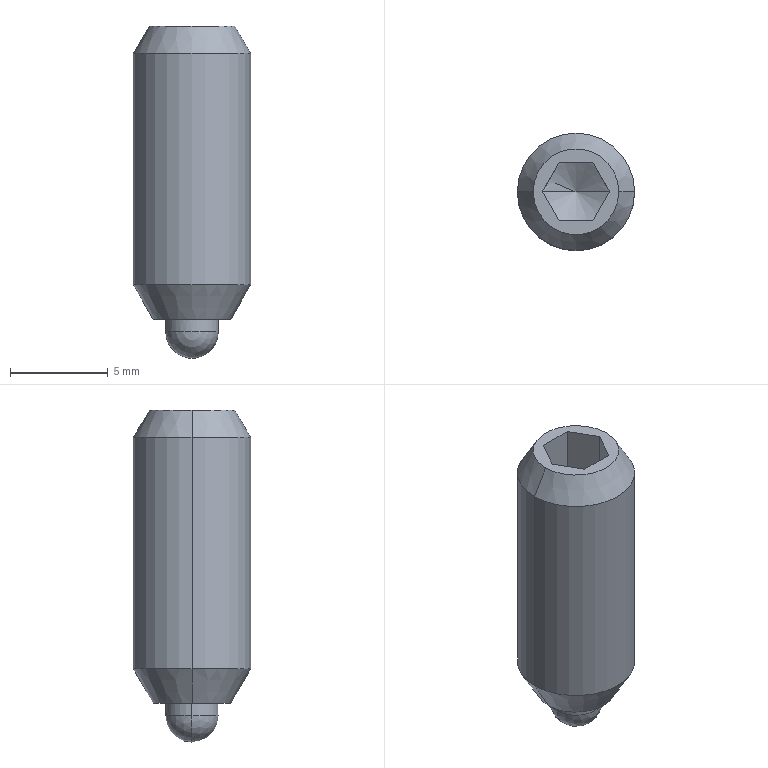Part | NX | features BREP 2 | 2 solids | 29 faces | box 6 x 6 x 17 mm | volume 380.172 mm3 | plane 11 | cylinder 8 | cone 8 | sphere 2 | commonest cylinder face diameters 3.5 x4 2.7 x2 6 x2
STEP:
#1=CARTESIAN_POINT('',(1.75,0.,5.8));
#2=VERTEX_POINT('',#1);
#3=CARTESIAN_POINT('',(1.75,0.,2.3));
#4=VERTEX_POINT('',#3);
#5=CARTESIAN_POINT('',(1.75,0.,4.05));
#6=DIRECTION('',(0.,0.,-1.));
#7=VECTOR('',#6,1000.);
#8=LINE('',#5,#7);
#9=EDGE_CURVE('',#2,#4,#8,.T.);
#10=ORIENTED_EDGE('',*,*,#9,.F.);
#11=CARTESIAN_POINT('',(-1.75,0.,5.8));
#12=VERTEX_POINT('',#11);
#13=CARTESIAN_POINT('',(0.,0.,5.8));
#14=DIRECTION('',(0.,0.,-1.));
#15=DIRECTION('',(1.,0.,0.));
#16=AXIS2_PLACEMENT_3D('',#13,#14,#15);
#17=CIRCLE('',#16,1.75);
#18=EDGE_CURVE('',#2,#12,#17,.T.);
#19=ORIENTED_EDGE('',*,*,#18,.T.);
#20=CARTESIAN_POINT('',(-1.75,0.,2.3));
#21=VERTEX_POINT('',#20);
#22=CARTESIAN_POINT('',(-1.75,0.,4.05));
#23=DIRECTION('',(0.,0.,1.));
#24=VECTOR('',#23,1000.);
#25=LINE('',#22,#24);
#26=EDGE_CURVE('',#21,#12,#25,.T.);
#27=ORIENTED_EDGE('',*,*,#26,.F.);
#28=CARTESIAN_POINT('',(0.,0.,2.3));
#29=DIRECTION('',(0.,0.,-1.));
#30=DIRECTION('',(1.,0.,0.));
#31=AXIS2_PLACEMENT_3D('',#28,#29,#30);
#32=CIRCLE('',#31,1.75);
#33=EDGE_CURVE('',#4,#21,#32,.T.);
#34=ORIENTED_EDGE('',*,*,#33,.F.);
#35=EDGE_LOOP('',(#10,#19,#27,#34));
#36=FACE_BOUND('',#35,.T.);
#37=CARTESIAN_POINT('',(0.,0.,4.05));
#38=DIRECTION('',(0.,0.,1.));
#39=DIRECTION('',(-1.,0.,0.));
#40=AXIS2_PLACEMENT_3D('',#37,#38,#39);
#41=CYLINDRICAL_SURFACE('',#40,1.75);
#42=ADVANCED_FACE('',(#36),#41,.T.);
#43=CARTESIAN_POINT('',(1.35,0.,1.35));
#44=VERTEX_POINT('',#43);
#45=CARTESIAN_POINT('',(-1.35,0.,1.35));
#46=VERTEX_POINT('',#45);
#47=CARTESIAN_POINT('',(0.,0.,1.35));
#48=DIRECTION('',(0.,1.,0.));
#49=DIRECTION('',(0.,0.,-1.));
#50=AXIS2_PLACEMENT_3D('',#47,#48,#49);
#51=CIRCLE('',#50,1.35);
#52=EDGE_CURVE('',#44,#46,#51,.T.);
#53=ORIENTED_EDGE('',*,*,#52,.F.);
#54=CARTESIAN_POINT('',(0.,0.,1.35));
#55=DIRECTION('',(0.,0.,-1.));
#56=DIRECTION('',(1.,0.,0.));
#57=AXIS2_PLACEMENT_3D('',#54,#55,#56);
#58=CIRCLE('',#57,1.35);
#59=EDGE_CURVE('',#44,#46,#58,.T.);
#60=ORIENTED_EDGE('',*,*,#59,.T.);
#61=EDGE_LOOP('',(#53,#60));
#62=FACE_BOUND('',#61,.T.);
#63=CARTESIAN_POINT('',(0.,0.,1.35));
#64=DIRECTION('',(0.,-1.,0.));
#65=DIRECTION('',(-1.,0.,0.));
#66=AXIS2_PLACEMENT_3D('',#63,#64,#65);
#67=SPHERICAL_SURFACE('',#66,1.35);
#68=ADVANCED_FACE('',(#62),#67,.T.);
#69=CARTESIAN_POINT('',(1.35,0.,2.3));
#70=VERTEX_POINT('',#69);
#71=CARTESIAN_POINT('',(1.35,0.,1.825));
#72=DIRECTION('',(0.,0.,-1.));
#73=VECTOR('',#72,1000.);
#74=LINE('',#71,#73);
#75=EDGE_CURVE('',#70,#44,#74,.T.);
#76=ORIENTED_EDGE('',*,*,#75,.F.);
#77=CARTESIAN_POINT('',(-1.35,0.,2.3));
#78=VERTEX_POINT('',#77);
#79=CARTESIAN_POINT('',(0.,0.,2.3));
#80=DIRECTION('',(0.,0.,-1.));
#81=DIRECTION('',(1.,0.,0.));
#82=AXIS2_PLACEMENT_3D('',#79,#80,#81);
#83=CIRCLE('',#82,1.35);
#84=EDGE_CURVE('',#70,#78,#83,.T.);
#85=ORIENTED_EDGE('',*,*,#84,.T.);
#86=CARTESIAN_POINT('',(-1.35,0.,1.825));
#87=DIRECTION('',(0.,0.,1.));
#88=VECTOR('',#87,1000.);
#89=LINE('',#86,#88);
#90=EDGE_CURVE('',#46,#78,#89,.T.);
#91=ORIENTED_EDGE('',*,*,#90,.F.);
#92=ORIENTED_EDGE('',*,*,#59,.F.);
#93=EDGE_LOOP('',(#76,#85,#91,#92));
#94=FACE_BOUND('',#93,.T.);
#95=CARTESIAN_POINT('',(0.,0.,1.825));
#96=DIRECTION('',(0.,0.,1.));
#97=DIRECTION('',(-1.,0.,0.));
#98=AXIS2_PLACEMENT_3D('',#95,#96,#97);
#99=CYLINDRICAL_SURFACE('',#98,1.35);
#100=ADVANCED_FACE('',(#94),#99,.T.);
#101=ORIENTED_EDGE('',*,*,#33,.T.);
#102=CARTESIAN_POINT('',(0.,0.,2.3));
#103=DIRECTION('',(0.,0.,-1.));
#104=DIRECTION('',(1.,0.,0.));
#105=AXIS2_PLACEMENT_3D('',#102,#103,#104);
#106=CIRCLE('',#105,1.75);
#107=EDGE_CURVE('',#21,#4,#106,.T.);
#108=ORIENTED_EDGE('',*,*,#107,.T.);
#109=EDGE_LOOP('',(#101,#108));
#110=FACE_BOUND('',#109,.T.);
#111=ORIENTED_EDGE('',*,*,#84,.F.);
#112=CARTESIAN_POINT('',(0.,0.,2.3));
#113=DIRECTION('',(0.,0.,-1.));
#114=DIRECTION('',(1.,0.,0.));
#115=AXIS2_PLACEMENT_3D('',#112,#113,#114);
#116=CIRCLE('',#115,1.35);
#117=EDGE_CURVE('',#78,#70,#116,.T.);
#118=ORIENTED_EDGE('',*,*,#117,.F.);
#119=EDGE_LOOP('',(#111,#118));
#120=FACE_BOUND('',#119,.T.);
#121=CARTESIAN_POINT('',(1.55,0.,2.3));
#122=DIRECTION('',(0.,0.,-1.));
#123=DIRECTION('',(0.,1.,0.));
#124=AXIS2_PLACEMENT_3D('',#121,#122,#123);
#125=PLANE('',#124);
#126=ADVANCED_FACE('',(#110,#120),#125,.T.);
#127=ORIENTED_EDGE('',*,*,#75,.T.);
#128=CARTESIAN_POINT('',(0.,0.,1.35));
#129=DIRECTION('',(0.,0.,-1.));
#130=DIRECTION('',(1.,0.,0.));
#131=AXIS2_PLACEMENT_3D('',#128,#129,#130);
#132=CIRCLE('',#131,1.35);
#133=EDGE_CURVE('',#46,#44,#132,.T.);
#134=ORIENTED_EDGE('',*,*,#133,.F.);
#135=ORIENTED_EDGE('',*,*,#90,.T.);
#136=ORIENTED_EDGE('',*,*,#117,.T.);
#137=EDGE_LOOP('',(#127,#134,#135,#136));
#138=FACE_BOUND('',#137,.T.);
#139=CARTESIAN_POINT('',(0.,0.,1.825));
#140=DIRECTION('',(0.,0.,1.));
#141=DIRECTION('',(-1.,0.,0.));
#142=AXIS2_PLACEMENT_3D('',#139,#140,#141);
#143=CYLINDRICAL_SURFACE('',#142,1.35);
#144=ADVANCED_FACE('',(#138),#143,.T.);
#145=ORIENTED_EDGE('',*,*,#52,.T.);
#146=ORIENTED_EDGE('',*,*,#133,.T.);
#147=EDGE_LOOP('',(#145,#146));
#148=FACE_BOUND('',#147,.T.);
#149=CARTESIAN_POINT('',(0.,0.,1.35));
#150=DIRECTION('',(0.,-1.,0.));
#151=DIRECTION('',(-1.,0.,0.));
#152=AXIS2_PLACEMENT_3D('',#149,#150,#151);
#153=SPHERICAL_SURFACE('',#152,1.35);
#154=ADVANCED_FACE('',(#148),#153,.T.);
#155=ORIENTED_EDGE('',*,*,#18,.F.);
#156=CARTESIAN_POINT('',(0.,0.,5.8));
#157=DIRECTION('',(0.,0.,-1.));
#158=DIRECTION('',(1.,0.,0.));
#159=AXIS2_PLACEMENT_3D('',#156,#157,#158);
#160=CIRCLE('',#159,1.75);
#161=EDGE_CURVE('',#12,#2,#160,.T.);
#162=ORIENTED_EDGE('',*,*,#161,.F.);
#163=EDGE_LOOP('',(#155,#162));
#164=FACE_BOUND('',#163,.T.);
#165=CARTESIAN_POINT('',(0.875,0.,5.8));
#166=DIRECTION('',(0.,0.,1.));
#167=DIRECTION('',(-1.,0.,0.));
#168=AXIS2_PLACEMENT_3D('',#165,#166,#167);
#169=PLANE('',#168);
#170=ADVANCED_FACE('',(#164),#169,.T.);
#171=ORIENTED_EDGE('',*,*,#9,.T.);
#172=ORIENTED_EDGE('',*,*,#107,.F.);
#173=ORIENTED_EDGE('',*,*,#26,.T.);
#174=ORIENTED_EDGE('',*,*,#161,.T.);
#175=EDGE_LOOP('',(#171,#172,#173,#174));
#176=FACE_BOUND('',#175,.T.);
#177=CARTESIAN_POINT('',(0.,0.,4.05));
#178=DIRECTION('',(0.,0.,1.));
#179=DIRECTION('',(-1.,0.,0.));
#180=AXIS2_PLACEMENT_3D('',#177,#178,#179);
#181=CYLINDRICAL_SURFACE('',#180,1.75);
#182=ADVANCED_FACE('',(#176),#181,.T.);
#183=CLOSED_SHELL('',(#42,#68,#100,#126,#144,#154,#170,#182));
#184=MANIFOLD_SOLID_BREP('',#183);
#185=CARTESIAN_POINT('',(-3.,0.,3.75));
#186=VERTEX_POINT('',#185);
#187=CARTESIAN_POINT('',(-1.99,0.,2.));
#188=VERTEX_POINT('',#187);
#189=CARTESIAN_POINT('',(-2.495,0.,2.875));
#190=DIRECTION('',(0.5,0.,-0.866));
#191=VECTOR('',#190,1000.);
#192=LINE('',#189,#191);
#193=EDGE_CURVE('',#186,#188,#192,.T.);
#194=ORIENTED_EDGE('',*,*,#193,.F.);
#195=CARTESIAN_POINT('',(3.,0.,3.75));
#196=VERTEX_POINT('',#195);
#197=CARTESIAN_POINT('',(0.,0.,3.75));
#198=DIRECTION('',(0.,0.,-1.));
#199=DIRECTION('',(-1.,0.,0.));
#200=AXIS2_PLACEMENT_3D('',#197,#198,#199);
#201=CIRCLE('',#200,3.);
#202=EDGE_CURVE('',#186,#196,#201,.T.);
#203=ORIENTED_EDGE('',*,*,#202,.T.);
#204=CARTESIAN_POINT('',(1.99,0.,2.));
#205=VERTEX_POINT('',#204);
#206=CARTESIAN_POINT('',(2.495,0.,2.875));
#207=DIRECTION('',(0.5,0.,0.866));
#208=VECTOR('',#207,1000.);
#209=LINE('',#206,#208);
#210=EDGE_CURVE('',#205,#196,#209,.T.);
#211=ORIENTED_EDGE('',*,*,#210,.F.);
#212=CARTESIAN_POINT('',(0.,0.,2.));
#213=DIRECTION('',(0.,0.,-1.));
#214=DIRECTION('',(-1.,0.,0.));
#215=AXIS2_PLACEMENT_3D('',#212,#213,#214);
#216=CIRCLE('',#215,1.99);
#217=EDGE_CURVE('',#188,#205,#216,.T.);
#218=ORIENTED_EDGE('',*,*,#217,.F.);
#219=EDGE_LOOP('',(#194,#203,#211,#218));
#220=FACE_BOUND('',#219,.T.);
#221=CARTESIAN_POINT('',(0.,0.,2.875));
#222=DIRECTION('',(0.,0.,1.));
#223=DIRECTION('',(1.,0.,0.));
#224=AXIS2_PLACEMENT_3D('',#221,#222,#223);
#225=CONICAL_SURFACE('',#224,2.495,0.5236);
#226=ADVANCED_FACE('',(#220),#225,.T.);
#227=CARTESIAN_POINT('',(-3.,0.,15.6));
#228=VERTEX_POINT('',#227);
#229=CARTESIAN_POINT('',(-3.,0.,9.675));
#230=DIRECTION('',(0.,0.,-1.));
#231=VECTOR('',#230,1000.);
#232=LINE('',#229,#231);
#233=EDGE_CURVE('',#228,#186,#232,.T.);
#234=ORIENTED_EDGE('',*,*,#233,.F.);
#235=CARTESIAN_POINT('',(3.,0.,15.6));
#236=VERTEX_POINT('',#235);
#237=CARTESIAN_POINT('',(0.,0.,15.6));
#238=DIRECTION('',(0.,0.,-1.));
#239=DIRECTION('',(-1.,0.,0.));
#240=AXIS2_PLACEMENT_3D('',#237,#238,#239);
#241=CIRCLE('',#240,3.);
#242=EDGE_CURVE('',#228,#236,#241,.T.);
#243=ORIENTED_EDGE('',*,*,#242,.T.);
#244=CARTESIAN_POINT('',(3.,0.,9.675));
#245=DIRECTION('',(0.,0.,1.));
#246=VECTOR('',#245,1000.);
#247=LINE('',#244,#246);
#248=EDGE_CURVE('',#196,#236,#247,.T.);
#249=ORIENTED_EDGE('',*,*,#248,.F.);
#250=ORIENTED_EDGE('',*,*,#202,.F.);
#251=EDGE_LOOP('',(#234,#243,#249,#250));
#252=FACE_BOUND('',#251,.T.);
#253=CARTESIAN_POINT('',(0.,0.,9.675));
#254=DIRECTION('',(0.,0.,1.));
#255=DIRECTION('',(1.,0.,0.));
#256=AXIS2_PLACEMENT_3D('',#253,#254,#255);
#257=CYLINDRICAL_SURFACE('',#256,3.);
#258=ADVANCED_FACE('',(#252),#257,.T.);
#259=CARTESIAN_POINT('',(-2.192,0.,17.));
#260=VERTEX_POINT('',#259);
#261=CARTESIAN_POINT('',(-2.596,0.,16.3));
#262=DIRECTION('',(-0.5,0.,-0.866));
#263=VECTOR('',#262,1000.);
#264=LINE('',#261,#263);
#265=EDGE_CURVE('',#260,#228,#264,.T.);
#266=ORIENTED_EDGE('',*,*,#265,.F.);
#267=CARTESIAN_POINT('',(2.192,0.,17.));
#268=VERTEX_POINT('',#267);
#269=CARTESIAN_POINT('',(0.,0.,17.));
#270=DIRECTION('',(0.,0.,-1.));
#271=DIRECTION('',(-1.,0.,0.));
#272=AXIS2_PLACEMENT_3D('',#269,#270,#271);
#273=CIRCLE('',#272,2.192);
#274=EDGE_CURVE('',#260,#268,#273,.T.);
#275=ORIENTED_EDGE('',*,*,#274,.T.);
#276=CARTESIAN_POINT('',(2.596,0.,16.3));
#277=DIRECTION('',(-0.5,0.,0.866));
#278=VECTOR('',#277,1000.);
#279=LINE('',#276,#278);
#280=EDGE_CURVE('',#236,#268,#279,.T.);
#281=ORIENTED_EDGE('',*,*,#280,.F.);
#282=ORIENTED_EDGE('',*,*,#242,.F.);
#283=EDGE_LOOP('',(#266,#275,#281,#282));
#284=FACE_BOUND('',#283,.T.);
#285=CARTESIAN_POINT('',(0.,0.,16.3));
#286=DIRECTION('',(0.,0.,-1.));
#287=DIRECTION('',(1.,0.,0.));
#288=AXIS2_PLACEMENT_3D('',#285,#286,#287);
#289=CONICAL_SURFACE('',#288,2.596,0.5236);
#290=ADVANCED_FACE('',(#284),#289,.T.);
#291=CARTESIAN_POINT('',(0.,0.,12.804));
#292=VERTEX_POINT('',#291);
#293=CARTESIAN_POINT('',(1.725,0.,13.8));
#294=VERTEX_POINT('',#293);
#295=CARTESIAN_POINT('',(0.8625,0.,13.302));
#296=DIRECTION('',(0.866,0.,0.5));
#297=VECTOR('',#296,1000.);
#298=LINE('',#295,#297);
#299=EDGE_CURVE('',#292,#294,#298,.T.);
#300=ORIENTED_EDGE('',*,*,#299,.F.);
#301=CARTESIAN_POINT('',(-1.725,0.,13.8));
#302=VERTEX_POINT('',#301);
#303=CARTESIAN_POINT('',(-0.8625,0.,13.302));
#304=DIRECTION('',(0.866,0.,-0.5));
#305=VECTOR('',#304,1000.);
#306=LINE('',#303,#305);
#307=EDGE_CURVE('',#302,#292,#306,.T.);
#308=ORIENTED_EDGE('',*,*,#307,.F.);
#309=CARTESIAN_POINT('',(-0.8625,-1.494,13.8));
#310=VERTEX_POINT('',#309);
#311=CARTESIAN_POINT('',(-1.725,0.,13.8));
#312=CARTESIAN_POINT('',(-1.294,-0.7469,13.551));
#313=CARTESIAN_POINT('',(-0.8625,-1.494,13.8));
#314=(BOUNDED_CURVE()B_SPLINE_CURVE(2,(#311,#312,#313),.UNSPECIFIED.,.F.,.F.)B_SPLINE_CURVE_WITH_KNOTS((3,3),(0.,1.),.PIECEWISE_BEZIER_KNOTS.)CURVE()GEOMETRIC_REPRESENTATION_ITEM()RATIONAL_B_SPLINE_CURVE((1.,1.155,1.))REPRESENTATION_ITEM(''));
#315=EDGE_CURVE('',#302,#310,#314,.T.);
#316=ORIENTED_EDGE('',*,*,#315,.T.);
#317=CARTESIAN_POINT('',(0.8625,-1.494,13.8));
#318=VERTEX_POINT('',#317);
#319=CARTESIAN_POINT('',(-0.8625,-1.494,13.8));
#320=CARTESIAN_POINT('',(0.,-1.494,13.551));
#321=CARTESIAN_POINT('',(0.8625,-1.494,13.8));
#322=(BOUNDED_CURVE()B_SPLINE_CURVE(2,(#319,#320,#321),.UNSPECIFIED.,.F.,.F.)B_SPLINE_CURVE_WITH_KNOTS((3,3),(0.,1.),.PIECEWISE_BEZIER_KNOTS.)CURVE()GEOMETRIC_REPRESENTATION_ITEM()RATIONAL_B_SPLINE_CURVE((1.,1.155,1.))REPRESENTATION_ITEM(''));
#323=EDGE_CURVE('',#310,#318,#322,.T.);
#324=ORIENTED_EDGE('',*,*,#323,.T.);
#325=CARTESIAN_POINT('',(0.8625,-1.494,13.8));
#326=CARTESIAN_POINT('',(1.294,-0.7469,13.551));
#327=CARTESIAN_POINT('',(1.725,0.,13.8));
#328=(BOUNDED_CURVE()B_SPLINE_CURVE(2,(#325,#326,#327),.UNSPECIFIED.,.F.,.F.)B_SPLINE_CURVE_WITH_KNOTS((3,3),(0.,1.),.PIECEWISE_BEZIER_KNOTS.)CURVE()GEOMETRIC_REPRESENTATION_ITEM()RATIONAL_B_SPLINE_CURVE((1.,1.155,1.))REPRESENTATION_ITEM(''));
#329=EDGE_CURVE('',#318,#294,#328,.T.);
#330=ORIENTED_EDGE('',*,*,#329,.T.);
#331=EDGE_LOOP('',(#300,#308,#316,#324,#330));
#332=FACE_BOUND('',#331,.T.);
#333=CARTESIAN_POINT('',(0.,0.,13.302));
#334=DIRECTION('',(0.,0.,1.));
#335=DIRECTION('',(1.,0.,0.));
#336=AXIS2_PLACEMENT_3D('',#333,#334,#335);
#337=CONICAL_SURFACE('',#336,0.8625,1.047);
#338=ADVANCED_FACE('',(#332),#337,.F.);
#339=CARTESIAN_POINT('',(-1.35,0.,2.));
#340=VERTEX_POINT('',#339);
#341=CARTESIAN_POINT('',(-1.75,0.,2.3));
#342=VERTEX_POINT('',#341);
#343=CARTESIAN_POINT('',(-1.55,0.,2.15));
#344=DIRECTION('',(-0.8,0.,0.6));
#345=VECTOR('',#344,1000.);
#346=LINE('',#343,#345);
#347=EDGE_CURVE('',#340,#342,#346,.T.);
#348=ORIENTED_EDGE('',*,*,#347,.F.);
#349=CARTESIAN_POINT('',(1.35,0.,2.));
#350=VERTEX_POINT('',#349);
#351=CARTESIAN_POINT('',(0.,0.,2.));
#352=DIRECTION('',(0.,0.,1.));
#353=DIRECTION('',(-1.,0.,0.));
#354=AXIS2_PLACEMENT_3D('',#351,#352,#353);
#355=CIRCLE('',#354,1.35);
#356=EDGE_CURVE('',#350,#340,#355,.T.);
#357=ORIENTED_EDGE('',*,*,#356,.F.);
#358=CARTESIAN_POINT('',(1.75,0.,2.3));
#359=VERTEX_POINT('',#358);
#360=CARTESIAN_POINT('',(1.55,0.,2.15));
#361=DIRECTION('',(-0.8,0.,-0.6));
#362=VECTOR('',#361,1000.);
#363=LINE('',#360,#362);
#364=EDGE_CURVE('',#359,#350,#363,.T.);
#365=ORIENTED_EDGE('',*,*,#364,.F.);
#366=CARTESIAN_POINT('',(0.,0.,2.3));
#367=DIRECTION('',(0.,0.,-1.));
#368=DIRECTION('',(-1.,0.,0.));
#369=AXIS2_PLACEMENT_3D('',#366,#367,#368);
#370=CIRCLE('',#369,1.75);
#371=EDGE_CURVE('',#342,#359,#370,.T.);
#372=ORIENTED_EDGE('',*,*,#371,.F.);
#373=EDGE_LOOP('',(#348,#357,#365,#372));
#374=FACE_BOUND('',#373,.T.);
#375=CARTESIAN_POINT('',(0.,0.,2.15));
#376=DIRECTION('',(0.,0.,1.));
#377=DIRECTION('',(1.,0.,0.));
#378=AXIS2_PLACEMENT_3D('',#375,#376,#377);
#379=CONICAL_SURFACE('',#378,1.55,0.9273);
#380=ADVANCED_FACE('',(#374),#379,.F.);
#381=CARTESIAN_POINT('',(-1.75,0.,5.8));
#382=VERTEX_POINT('',#381);
#383=CARTESIAN_POINT('',(-1.75,0.,4.05));
#384=DIRECTION('',(0.,0.,1.));
#385=VECTOR('',#384,1000.);
#386=LINE('',#383,#385);
#387=EDGE_CURVE('',#342,#382,#386,.T.);
#388=ORIENTED_EDGE('',*,*,#387,.F.);
#389=ORIENTED_EDGE('',*,*,#371,.T.);
#390=CARTESIAN_POINT('',(1.75,0.,5.8));
#391=VERTEX_POINT('',#390);
#392=CARTESIAN_POINT('',(1.75,0.,4.05));
#393=DIRECTION('',(0.,0.,-1.));
#394=VECTOR('',#393,1000.);
#395=LINE('',#392,#394);
#396=EDGE_CURVE('',#391,#359,#395,.T.);
#397=ORIENTED_EDGE('',*,*,#396,.F.);
#398=CARTESIAN_POINT('',(0.,0.,5.8));
#399=DIRECTION('',(0.,0.,-1.));
#400=DIRECTION('',(-1.,0.,0.));
#401=AXIS2_PLACEMENT_3D('',#398,#399,#400);
#402=CIRCLE('',#401,1.75);
#403=EDGE_CURVE('',#382,#391,#402,.T.);
#404=ORIENTED_EDGE('',*,*,#403,.F.);
#405=EDGE_LOOP('',(#388,#389,#397,#404));
#406=FACE_BOUND('',#405,.T.);
#407=CARTESIAN_POINT('',(0.,0.,4.05));
#408=DIRECTION('',(0.,0.,1.));
#409=DIRECTION('',(1.,0.,0.));
#410=AXIS2_PLACEMENT_3D('',#407,#408,#409);
#411=CYLINDRICAL_SURFACE('',#410,1.75);
#412=ADVANCED_FACE('',(#406),#411,.F.);
#413=ORIENTED_EDGE('',*,*,#323,.F.);
#414=CARTESIAN_POINT('',(-0.8625,-1.494,17.));
#415=VERTEX_POINT('',#414);
#416=CARTESIAN_POINT('',(-0.8625,-1.494,15.4));
#417=DIRECTION('',(0.,0.,1.));
#418=VECTOR('',#417,1000.);
#419=LINE('',#416,#418);
#420=EDGE_CURVE('',#310,#415,#419,.T.);
#421=ORIENTED_EDGE('',*,*,#420,.T.);
#422=CARTESIAN_POINT('',(0.8625,-1.494,17.));
#423=VERTEX_POINT('',#422);
#424=CARTESIAN_POINT('',(-0.4313,-1.494,17.));
#425=DIRECTION('',(-1.,0.,0.));
#426=VECTOR('',#425,1000.);
#427=LINE('',#424,#426);
#428=EDGE_CURVE('',#423,#415,#427,.T.);
#429=ORIENTED_EDGE('',*,*,#428,.F.);
#430=CARTESIAN_POINT('',(0.8625,-1.494,15.4));
#431=DIRECTION('',(0.,0.,1.));
#432=VECTOR('',#431,1000.);
#433=LINE('',#430,#432);
#434=EDGE_CURVE('',#318,#423,#433,.T.);
#435=ORIENTED_EDGE('',*,*,#434,.F.);
#436=EDGE_LOOP('',(#413,#421,#429,#435));
#437=FACE_BOUND('',#436,.T.);
#438=CARTESIAN_POINT('',(-0.8625,-1.494,17.));
#439=DIRECTION('',(0.,-1.,0.));
#440=DIRECTION('',(0.,0.,1.));
#441=AXIS2_PLACEMENT_3D('',#438,#439,#440);
#442=PLANE('',#441);
#443=ADVANCED_FACE('',(#437),#442,.F.);
#444=ORIENTED_EDGE('',*,*,#315,.F.);
#445=CARTESIAN_POINT('',(-1.725,0.,17.));
#446=VERTEX_POINT('',#445);
#447=CARTESIAN_POINT('',(-1.725,0.,15.4));
#448=DIRECTION('',(0.,0.,1.));
#449=VECTOR('',#448,1000.);
#450=LINE('',#447,#449);
#451=EDGE_CURVE('',#302,#446,#450,.T.);
#452=ORIENTED_EDGE('',*,*,#451,.T.);
#453=CARTESIAN_POINT('',(-1.509,-0.3735,17.));
#454=DIRECTION('',(-0.5,0.866,0.));
#455=VECTOR('',#454,1000.);
#456=LINE('',#453,#455);
#457=EDGE_CURVE('',#415,#446,#456,.T.);
#458=ORIENTED_EDGE('',*,*,#457,.F.);
#459=ORIENTED_EDGE('',*,*,#420,.F.);
#460=EDGE_LOOP('',(#444,#452,#458,#459));
#461=FACE_BOUND('',#460,.T.);
#462=CARTESIAN_POINT('',(-1.725,0.,17.));
#463=DIRECTION('',(-0.866,-0.5,0.));
#464=DIRECTION('',(0.5,-0.866,0.));
#465=AXIS2_PLACEMENT_3D('',#462,#463,#464);
#466=PLANE('',#465);
#467=ADVANCED_FACE('',(#461),#466,.F.);
#468=CARTESIAN_POINT('',(-0.8625,1.494,13.8));
#469=VERTEX_POINT('',#468);
#470=CARTESIAN_POINT('',(-0.8625,1.494,13.8));
#471=CARTESIAN_POINT('',(-1.294,0.7469,13.551));
#472=CARTESIAN_POINT('',(-1.725,0.,13.8));
#473=(BOUNDED_CURVE()B_SPLINE_CURVE(2,(#470,#471,#472),.UNSPECIFIED.,.F.,.F.)B_SPLINE_CURVE_WITH_KNOTS((3,3),(0.,1.),.PIECEWISE_BEZIER_KNOTS.)CURVE()GEOMETRIC_REPRESENTATION_ITEM()RATIONAL_B_SPLINE_CURVE((1.,1.155,1.))REPRESENTATION_ITEM(''));
#474=EDGE_CURVE('',#469,#302,#473,.T.);
#475=ORIENTED_EDGE('',*,*,#474,.F.);
#476=CARTESIAN_POINT('',(-0.8625,1.494,17.));
#477=VERTEX_POINT('',#476);
#478=CARTESIAN_POINT('',(-0.8625,1.494,15.4));
#479=DIRECTION('',(0.,0.,1.));
#480=VECTOR('',#479,1000.);
#481=LINE('',#478,#480);
#482=EDGE_CURVE('',#469,#477,#481,.T.);
#483=ORIENTED_EDGE('',*,*,#482,.T.);
#484=CARTESIAN_POINT('',(-1.078,1.12,17.));
#485=DIRECTION('',(0.5,0.866,0.));
#486=VECTOR('',#485,1000.);
#487=LINE('',#484,#486);
#488=EDGE_CURVE('',#446,#477,#487,.T.);
#489=ORIENTED_EDGE('',*,*,#488,.F.);
#490=ORIENTED_EDGE('',*,*,#451,.F.);
#491=EDGE_LOOP('',(#475,#483,#489,#490));
#492=FACE_BOUND('',#491,.T.);
#493=CARTESIAN_POINT('',(-0.8625,1.494,17.));
#494=DIRECTION('',(-0.866,0.5,0.));
#495=DIRECTION('',(0.,0.,-1.));
#496=AXIS2_PLACEMENT_3D('',#493,#494,#495);
#497=PLANE('',#496);
#498=ADVANCED_FACE('',(#492),#497,.F.);
#499=CARTESIAN_POINT('',(0.8625,1.494,13.8));
#500=VERTEX_POINT('',#499);
#501=CARTESIAN_POINT('',(0.8625,1.494,13.8));
#502=CARTESIAN_POINT('',(0.,1.494,13.551));
#503=CARTESIAN_POINT('',(-0.8625,1.494,13.8));
#504=(BOUNDED_CURVE()B_SPLINE_CURVE(2,(#501,#502,#503),.UNSPECIFIED.,.F.,.F.)B_SPLINE_CURVE_WITH_KNOTS((3,3),(0.,1.),.PIECEWISE_BEZIER_KNOTS.)CURVE()GEOMETRIC_REPRESENTATION_ITEM()RATIONAL_B_SPLINE_CURVE((1.,1.155,1.))REPRESENTATION_ITEM(''));
#505=EDGE_CURVE('',#500,#469,#504,.T.);
#506=ORIENTED_EDGE('',*,*,#505,.F.);
#507=CARTESIAN_POINT('',(0.8625,1.494,17.));
#508=VERTEX_POINT('',#507);
#509=CARTESIAN_POINT('',(0.8625,1.494,15.4));
#510=DIRECTION('',(0.,0.,-1.));
#511=VECTOR('',#510,1000.);
#512=LINE('',#509,#511);
#513=EDGE_CURVE('',#508,#500,#512,.T.);
#514=ORIENTED_EDGE('',*,*,#513,.F.);
#515=CARTESIAN_POINT('',(0.4312,1.494,17.));
#516=DIRECTION('',(1.,0.,0.));
#517=VECTOR('',#516,1000.);
#518=LINE('',#515,#517);
#519=EDGE_CURVE('',#477,#508,#518,.T.);
#520=ORIENTED_EDGE('',*,*,#519,.F.);
#521=ORIENTED_EDGE('',*,*,#482,.F.);
#522=EDGE_LOOP('',(#506,#514,#520,#521));
#523=FACE_BOUND('',#522,.T.);
#524=CARTESIAN_POINT('',(0.8625,1.494,17.));
#525=DIRECTION('',(0.,1.,0.));
#526=DIRECTION('',(-1.,0.,0.));
#527=AXIS2_PLACEMENT_3D('',#524,#525,#526);
#528=PLANE('',#527);
#529=ADVANCED_FACE('',(#523),#528,.F.);
#530=ORIENTED_EDGE('',*,*,#329,.F.);
#531=ORIENTED_EDGE('',*,*,#434,.T.);
#532=CARTESIAN_POINT('',(1.725,0.,17.));
#533=VERTEX_POINT('',#532);
#534=CARTESIAN_POINT('',(1.078,-1.12,17.));
#535=DIRECTION('',(-0.5,-0.866,0.));
#536=VECTOR('',#535,1000.);
#537=LINE('',#534,#536);
#538=EDGE_CURVE('',#533,#423,#537,.T.);
#539=ORIENTED_EDGE('',*,*,#538,.F.);
#540=CARTESIAN_POINT('',(1.725,0.,15.4));
#541=DIRECTION('',(0.,0.,1.));
#542=VECTOR('',#541,1000.);
#543=LINE('',#540,#542);
#544=EDGE_CURVE('',#294,#533,#543,.T.);
#545=ORIENTED_EDGE('',*,*,#544,.F.);
#546=EDGE_LOOP('',(#530,#531,#539,#545));
#547=FACE_BOUND('',#546,.T.);
#548=CARTESIAN_POINT('',(0.8625,-1.494,17.));
#549=DIRECTION('',(0.866,-0.5,0.));
#550=DIRECTION('',(0.,0.,1.));
#551=AXIS2_PLACEMENT_3D('',#548,#549,#550);
#552=PLANE('',#551);
#553=ADVANCED_FACE('',(#547),#552,.F.);
#554=CARTESIAN_POINT('',(1.725,0.,13.8));
#555=CARTESIAN_POINT('',(1.294,0.7469,13.551));
#556=CARTESIAN_POINT('',(0.8625,1.494,13.8));
#557=(BOUNDED_CURVE()B_SPLINE_CURVE(2,(#554,#555,#556),.UNSPECIFIED.,.F.,.F.)B_SPLINE_CURVE_WITH_KNOTS((3,3),(0.,1.),.PIECEWISE_BEZIER_KNOTS.)CURVE()GEOMETRIC_REPRESENTATION_ITEM()RATIONAL_B_SPLINE_CURVE((1.,1.155,1.))REPRESENTATION_ITEM(''));
#558=EDGE_CURVE('',#294,#500,#557,.T.);
#559=ORIENTED_EDGE('',*,*,#558,.F.);
#560=ORIENTED_EDGE('',*,*,#544,.T.);
#561=CARTESIAN_POINT('',(1.509,0.3735,17.));
#562=DIRECTION('',(0.5,-0.866,0.));
#563=VECTOR('',#562,1000.);
#564=LINE('',#561,#563);
#565=EDGE_CURVE('',#508,#533,#564,.T.);
#566=ORIENTED_EDGE('',*,*,#565,.F.);
#567=ORIENTED_EDGE('',*,*,#513,.T.);
#568=EDGE_LOOP('',(#559,#560,#566,#567));
#569=FACE_BOUND('',#568,.T.);
#570=CARTESIAN_POINT('',(1.725,0.,17.));
#571=DIRECTION('',(0.866,0.5,0.));
#572=DIRECTION('',(0.,0.,1.));
#573=AXIS2_PLACEMENT_3D('',#570,#571,#572);
#574=PLANE('',#573);
#575=ADVANCED_FACE('',(#569),#574,.F.);
#576=ORIENTED_EDGE('',*,*,#403,.T.);
#577=CARTESIAN_POINT('',(0.,0.,5.8));
#578=DIRECTION('',(0.,0.,-1.));
#579=DIRECTION('',(-1.,0.,0.));
#580=AXIS2_PLACEMENT_3D('',#577,#578,#579);
#581=CIRCLE('',#580,1.75);
#582=EDGE_CURVE('',#391,#382,#581,.T.);
#583=ORIENTED_EDGE('',*,*,#582,.T.);
#584=EDGE_LOOP('',(#576,#583));
#585=FACE_BOUND('',#584,.T.);
#586=CARTESIAN_POINT('',(-0.875,0.,5.8));
#587=DIRECTION('',(0.,0.,1.));
#588=DIRECTION('',(-1.,0.,0.));
#589=AXIS2_PLACEMENT_3D('',#586,#587,#588);
#590=PLANE('',#589);
#591=ADVANCED_FACE('',(#585),#590,.F.);
#592=ORIENTED_EDGE('',*,*,#387,.T.);
#593=ORIENTED_EDGE('',*,*,#582,.F.);
#594=ORIENTED_EDGE('',*,*,#396,.T.);
#595=CARTESIAN_POINT('',(0.,0.,2.3));
#596=DIRECTION('',(0.,0.,-1.));
#597=DIRECTION('',(-1.,0.,0.));
#598=AXIS2_PLACEMENT_3D('',#595,#596,#597);
#599=CIRCLE('',#598,1.75);
#600=EDGE_CURVE('',#359,#342,#599,.T.);
#601=ORIENTED_EDGE('',*,*,#600,.T.);
#602=EDGE_LOOP('',(#592,#593,#594,#601));
#603=FACE_BOUND('',#602,.T.);
#604=CARTESIAN_POINT('',(0.,0.,4.05));
#605=DIRECTION('',(0.,0.,1.));
#606=DIRECTION('',(1.,0.,0.));
#607=AXIS2_PLACEMENT_3D('',#604,#605,#606);
#608=CYLINDRICAL_SURFACE('',#607,1.75);
#609=ADVANCED_FACE('',(#603),#608,.F.);
#610=ORIENTED_EDGE('',*,*,#347,.T.);
#611=ORIENTED_EDGE('',*,*,#600,.F.);
#612=ORIENTED_EDGE('',*,*,#364,.T.);
#613=CARTESIAN_POINT('',(0.,0.,2.));
#614=DIRECTION('',(0.,0.,1.));
#615=DIRECTION('',(-1.,0.,0.));
#616=AXIS2_PLACEMENT_3D('',#613,#614,#615);
#617=CIRCLE('',#616,1.35);
#618=EDGE_CURVE('',#340,#350,#617,.T.);
#619=ORIENTED_EDGE('',*,*,#618,.F.);
#620=EDGE_LOOP('',(#610,#611,#612,#619));
#621=FACE_BOUND('',#620,.T.);
#622=CARTESIAN_POINT('',(0.,0.,2.15));
#623=DIRECTION('',(0.,0.,1.));
#624=DIRECTION('',(1.,0.,0.));
#625=AXIS2_PLACEMENT_3D('',#622,#623,#624);
#626=CONICAL_SURFACE('',#625,1.55,0.9273);
#627=ADVANCED_FACE('',(#621),#626,.F.);
#628=ORIENTED_EDGE('',*,*,#299,.T.);
#629=ORIENTED_EDGE('',*,*,#558,.T.);
#630=ORIENTED_EDGE('',*,*,#505,.T.);
#631=ORIENTED_EDGE('',*,*,#474,.T.);
#632=ORIENTED_EDGE('',*,*,#307,.T.);
#633=EDGE_LOOP('',(#628,#629,#630,#631,#632));
#634=FACE_BOUND('',#633,.T.);
#635=CARTESIAN_POINT('',(0.,0.,13.302));
#636=DIRECTION('',(0.,0.,1.));
#637=DIRECTION('',(1.,0.,0.));
#638=AXIS2_PLACEMENT_3D('',#635,#636,#637);
#639=CONICAL_SURFACE('',#638,0.8625,1.047);
#640=ADVANCED_FACE('',(#634),#639,.F.);
#641=ORIENTED_EDGE('',*,*,#274,.F.);
#642=CARTESIAN_POINT('',(0.,0.,17.));
#643=DIRECTION('',(0.,0.,-1.));
#644=DIRECTION('',(-1.,0.,0.));
#645=AXIS2_PLACEMENT_3D('',#642,#643,#644);
#646=CIRCLE('',#645,2.192);
#647=EDGE_CURVE('',#268,#260,#646,.T.);
#648=ORIENTED_EDGE('',*,*,#647,.F.);
#649=EDGE_LOOP('',(#641,#648));
#650=FACE_BOUND('',#649,.T.);
#651=ORIENTED_EDGE('',*,*,#519,.T.);
#652=ORIENTED_EDGE('',*,*,#565,.T.);
#653=ORIENTED_EDGE('',*,*,#538,.T.);
#654=ORIENTED_EDGE('',*,*,#428,.T.);
#655=ORIENTED_EDGE('',*,*,#457,.T.);
#656=ORIENTED_EDGE('',*,*,#488,.T.);
#657=EDGE_LOOP('',(#651,#652,#653,#654,#655,#656));
#658=FACE_BOUND('',#657,.T.);
#659=CARTESIAN_POINT('',(-1.958,0.,17.));
#660=DIRECTION('',(0.,0.,1.));
#661=DIRECTION('',(-1.,0.,0.));
#662=AXIS2_PLACEMENT_3D('',#659,#660,#661);
#663=PLANE('',#662);
#664=ADVANCED_FACE('',(#650,#658),#663,.T.);
#665=ORIENTED_EDGE('',*,*,#265,.T.);
#666=CARTESIAN_POINT('',(0.,0.,15.6));
#667=DIRECTION('',(0.,0.,-1.));
#668=DIRECTION('',(-1.,0.,0.));
#669=AXIS2_PLACEMENT_3D('',#666,#667,#668);
#670=CIRCLE('',#669,3.);
#671=EDGE_CURVE('',#236,#228,#670,.T.);
#672=ORIENTED_EDGE('',*,*,#671,.F.);
#673=ORIENTED_EDGE('',*,*,#280,.T.);
#674=ORIENTED_EDGE('',*,*,#647,.T.);
#675=EDGE_LOOP('',(#665,#672,#673,#674));
#676=FACE_BOUND('',#675,.T.);
#677=CARTESIAN_POINT('',(0.,0.,16.3));
#678=DIRECTION('',(0.,0.,-1.));
#679=DIRECTION('',(1.,0.,0.));
#680=AXIS2_PLACEMENT_3D('',#677,#678,#679);
#681=CONICAL_SURFACE('',#680,2.596,0.5236);
#682=ADVANCED_FACE('',(#676),#681,.T.);
#683=ORIENTED_EDGE('',*,*,#233,.T.);
#684=CARTESIAN_POINT('',(0.,0.,3.75));
#685=DIRECTION('',(0.,0.,-1.));
#686=DIRECTION('',(-1.,0.,0.));
#687=AXIS2_PLACEMENT_3D('',#684,#685,#686);
#688=CIRCLE('',#687,3.);
#689=EDGE_CURVE('',#196,#186,#688,.T.);
#690=ORIENTED_EDGE('',*,*,#689,.F.);
#691=ORIENTED_EDGE('',*,*,#248,.T.);
#692=ORIENTED_EDGE('',*,*,#671,.T.);
#693=EDGE_LOOP('',(#683,#690,#691,#692));
#694=FACE_BOUND('',#693,.T.);
#695=CARTESIAN_POINT('',(0.,0.,9.675));
#696=DIRECTION('',(0.,0.,1.));
#697=DIRECTION('',(1.,0.,0.));
#698=AXIS2_PLACEMENT_3D('',#695,#696,#697);
#699=CYLINDRICAL_SURFACE('',#698,3.);
#700=ADVANCED_FACE('',(#694),#699,.T.);
#701=ORIENTED_EDGE('',*,*,#193,.T.);
#702=CARTESIAN_POINT('',(0.,0.,2.));
#703=DIRECTION('',(0.,0.,-1.));
#704=DIRECTION('',(-1.,0.,0.));
#705=AXIS2_PLACEMENT_3D('',#702,#703,#704);
#706=CIRCLE('',#705,1.99);
#707=EDGE_CURVE('',#205,#188,#706,.T.);
#708=ORIENTED_EDGE('',*,*,#707,.F.);
#709=ORIENTED_EDGE('',*,*,#210,.T.);
#710=ORIENTED_EDGE('',*,*,#689,.T.);
#711=EDGE_LOOP('',(#701,#708,#709,#710));
#712=FACE_BOUND('',#711,.T.);
#713=CARTESIAN_POINT('',(0.,0.,2.875));
#714=DIRECTION('',(0.,0.,1.));
#715=DIRECTION('',(1.,0.,0.));
#716=AXIS2_PLACEMENT_3D('',#713,#714,#715);
#717=CONICAL_SURFACE('',#716,2.495,0.5236);
#718=ADVANCED_FACE('',(#712),#717,.T.);
#719=ORIENTED_EDGE('',*,*,#217,.T.);
#720=ORIENTED_EDGE('',*,*,#707,.T.);
#721=EDGE_LOOP('',(#719,#720));
#722=FACE_BOUND('',#721,.T.);
#723=ORIENTED_EDGE('',*,*,#618,.T.);
#724=ORIENTED_EDGE('',*,*,#356,.T.);
#725=EDGE_LOOP('',(#723,#724));
#726=FACE_BOUND('',#725,.T.);
#727=CARTESIAN_POINT('',(-0.9948,0.,2.));
#728=DIRECTION('',(0.,0.,-1.));
#729=DIRECTION('',(0.,1.,0.));
#730=AXIS2_PLACEMENT_3D('',#727,#728,#729);
#731=PLANE('',#730);
#732=ADVANCED_FACE('',(#722,#726),#731,.T.);
#733=CLOSED_SHELL('',(#226,#258,#290,#338,#380,#412,#443,#467,#498,#529,#553,#575,#591,#609,#627,#640,#664,#682,#700,#718,#732));
#734=MANIFOLD_SOLID_BREP('',#733);
#735=(LENGTH_UNIT()NAMED_UNIT(*)SI_UNIT(.MILLI.,.METRE.));
#736=UNCERTAINTY_MEASURE_WITH_UNIT(LENGTH_MEASURE(0.00001),#735,'','');
#737=(NAMED_UNIT(*)PLANE_ANGLE_UNIT()SI_UNIT($,.RADIAN.));
#738=(NAMED_UNIT(*)SI_UNIT($,.STERADIAN.)SOLID_ANGLE_UNIT());
#739=(GEOMETRIC_REPRESENTATION_CONTEXT(3)GLOBAL_UNCERTAINTY_ASSIGNED_CONTEXT((#736))GLOBAL_UNIT_ASSIGNED_CONTEXT((#735,#737,#738))REPRESENTATION_CONTEXT('',''));
#740=ADVANCED_BREP_SHAPE_REPRESENTATION('',(#184,#734),#739);